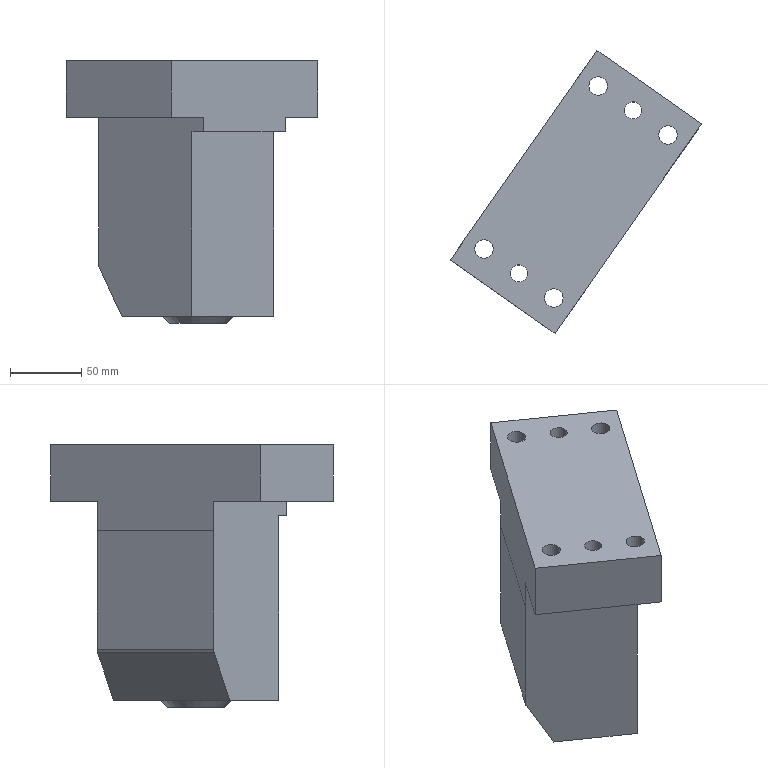Part | NX | features solid 2 | 1 solid | 34 faces | box 176.967 x 199.069 x 185 mm | volume 1701665 mm3 | plane 20 | cylinder 12 | cone 2 | commonest cylinder face diameters 20 x5 13 x4 12 x2 10 x1
STEP:
#1=CARTESIAN_POINT('',(-203.117,147.18,-70.));
#2=VERTEX_POINT('',#1);
#3=CARTESIAN_POINT('',(-196.617,147.18,-70.));
#4=DIRECTION('',(0.,0.,-1.));
#5=DIRECTION('',(-1.,0.,0.));
#6=AXIS2_PLACEMENT_3D('',#3,#4,#5);
#7=CIRCLE('',#6,6.5);
#8=EDGE_CURVE('',#2,#2,#7,.T.);
#9=ORIENTED_EDGE('',*,*,#8,.T.);
#10=EDGE_LOOP('',(#9));
#11=FACE_BOUND('',#10,.T.);
#12=CARTESIAN_POINT('',(-252.266,181.595,-70.));
#13=VERTEX_POINT('',#12);
#14=CARTESIAN_POINT('',(-245.766,181.595,-70.));
#15=DIRECTION('',(0.,0.,-1.));
#16=DIRECTION('',(-1.,0.,0.));
#17=AXIS2_PLACEMENT_3D('',#14,#15,#16);
#18=CIRCLE('',#17,6.5);
#19=EDGE_CURVE('',#13,#13,#18,.T.);
#20=ORIENTED_EDGE('',*,*,#19,.T.);
#21=EDGE_LOOP('',(#20));
#22=FACE_BOUND('',#21,.T.);
#23=CARTESIAN_POINT('',(-283.417,32.499,-70.));
#24=VERTEX_POINT('',#23);
#25=CARTESIAN_POINT('',(-276.917,32.499,-70.));
#26=DIRECTION('',(0.,0.,-1.));
#27=DIRECTION('',(-1.,0.,0.));
#28=AXIS2_PLACEMENT_3D('',#25,#26,#27);
#29=CIRCLE('',#28,6.5);
#30=EDGE_CURVE('',#24,#24,#29,.T.);
#31=ORIENTED_EDGE('',*,*,#30,.T.);
#32=EDGE_LOOP('',(#31));
#33=FACE_BOUND('',#32,.T.);
#34=CARTESIAN_POINT('',(-332.566,66.914,-70.));
#35=VERTEX_POINT('',#34);
#36=CARTESIAN_POINT('',(-326.066,66.914,-70.));
#37=DIRECTION('',(0.,0.,-1.));
#38=DIRECTION('',(-1.,0.,0.));
#39=AXIS2_PLACEMENT_3D('',#36,#37,#38);
#40=CIRCLE('',#39,6.5);
#41=EDGE_CURVE('',#35,#35,#40,.T.);
#42=ORIENTED_EDGE('',*,*,#41,.T.);
#43=EDGE_LOOP('',(#42));
#44=FACE_BOUND('',#43,.T.);
#45=CARTESIAN_POINT('',(-246.581,206.581,-70.));
#46=VERTEX_POINT('',#45);
#47=CARTESIAN_POINT('',(-349.824,59.134,-70.));
#48=VERTEX_POINT('',#47);
#49=CARTESIAN_POINT('',(-326.881,91.9,-70.));
#50=DIRECTION('',(-0.5736,-0.8192,0.));
#51=VECTOR('',#50,1000.);
#52=LINE('',#49,#51);
#53=EDGE_CURVE('',#46,#48,#52,.T.);
#54=ORIENTED_EDGE('',*,*,#53,.T.);
#55=CARTESIAN_POINT('',(-276.102,7.513,-70.));
#56=VERTEX_POINT('',#55);
#57=CARTESIAN_POINT('',(-349.825,59.134,-70.));
#58=DIRECTION('',(0.8192,-0.5736,0.));
#59=VECTOR('',#58,1000.);
#60=LINE('',#57,#59);
#61=EDGE_CURVE('',#48,#56,#60,.T.);
#62=ORIENTED_EDGE('',*,*,#61,.T.);
#63=CARTESIAN_POINT('',(-172.858,154.96,-70.));
#64=VERTEX_POINT('',#63);
#65=CARTESIAN_POINT('',(-253.159,40.279,-70.));
#66=DIRECTION('',(0.5736,0.8192,0.));
#67=VECTOR('',#66,1000.);
#68=LINE('',#65,#67);
#69=EDGE_CURVE('',#56,#64,#68,.T.);
#70=ORIENTED_EDGE('',*,*,#69,.T.);
#71=CARTESIAN_POINT('',(-263.134,218.172,-70.));
#72=DIRECTION('',(0.8192,-0.5736,0.));
#73=VECTOR('',#72,1000.);
#74=LINE('',#71,#73);
#75=EDGE_CURVE('',#46,#64,#74,.T.);
#76=ORIENTED_EDGE('',*,*,#75,.F.);
#77=EDGE_LOOP('',(#54,#62,#70,#76));
#78=FACE_BOUND('',#77,.T.);
#79=CARTESIAN_POINT('',(-227.191,164.388,-70.));
#80=VERTEX_POINT('',#79);
#81=CARTESIAN_POINT('',(-221.191,164.388,-70.));
#82=DIRECTION('',(0.,0.,-1.));
#83=DIRECTION('',(-1.,0.,0.));
#84=AXIS2_PLACEMENT_3D('',#81,#82,#83);
#85=CIRCLE('',#84,6.);
#86=EDGE_CURVE('',#80,#80,#85,.T.);
#87=ORIENTED_EDGE('',*,*,#86,.T.);
#88=EDGE_LOOP('',(#87));
#89=FACE_BOUND('',#88,.T.);
#90=CARTESIAN_POINT('',(-307.492,49.706,-70.));
#91=VERTEX_POINT('',#90);
#92=CARTESIAN_POINT('',(-301.492,49.706,-70.));
#93=DIRECTION('',(0.,0.,-1.));
#94=DIRECTION('',(-1.,0.,0.));
#95=AXIS2_PLACEMENT_3D('',#92,#93,#94);
#96=CIRCLE('',#95,6.);
#97=EDGE_CURVE('',#91,#91,#96,.F.);
#98=ORIENTED_EDGE('',*,*,#97,.F.);
#99=EDGE_LOOP('',(#98));
#100=FACE_BOUND('',#99,.T.);
#101=CARTESIAN_POINT('',(-343.435,103.491,-70.));
#102=DIRECTION('',(0.,0.,1.));
#103=DIRECTION('',(0.5736,0.8192,0.));
#104=AXIS2_PLACEMENT_3D('',#101,#102,#103);
#105=PLANE('',#104);
#106=ADVANCED_FACE('',(#11,#22,#33,#44,#78,#89,#100),#105,.T.);
#107=CARTESIAN_POINT('',(-286.917,32.499,-110.));
#108=VERTEX_POINT('',#107);
#109=CARTESIAN_POINT('',(-276.917,32.499,-110.));
#110=DIRECTION('',(0.,0.,-1.));
#111=DIRECTION('',(-1.,0.,0.));
#112=AXIS2_PLACEMENT_3D('',#109,#110,#111);
#113=CIRCLE('',#112,10.);
#114=EDGE_CURVE('',#108,#108,#113,.T.);
#115=ORIENTED_EDGE('',*,*,#114,.F.);
#116=EDGE_LOOP('',(#115));
#117=FACE_BOUND('',#116,.T.);
#118=CARTESIAN_POINT('',(-336.066,66.914,-110.));
#119=VERTEX_POINT('',#118);
#120=CARTESIAN_POINT('',(-326.066,66.914,-110.));
#121=DIRECTION('',(0.,0.,-1.));
#122=DIRECTION('',(-1.,0.,0.));
#123=AXIS2_PLACEMENT_3D('',#120,#121,#122);
#124=CIRCLE('',#123,10.);
#125=EDGE_CURVE('',#119,#119,#124,.T.);
#126=ORIENTED_EDGE('',*,*,#125,.F.);
#127=EDGE_LOOP('',(#126));
#128=FACE_BOUND('',#127,.T.);
#129=CARTESIAN_POINT('',(-326.881,91.9,-110.));
#130=VERTEX_POINT('',#129);
#131=CARTESIAN_POINT('',(-253.159,40.279,-110.));
#132=VERTEX_POINT('',#131);
#133=CARTESIAN_POINT('',(-326.882,91.9,-110.));
#134=DIRECTION('',(-0.8192,0.5736,0.));
#135=VECTOR('',#134,1000.);
#136=LINE('',#133,#135);
#137=EDGE_CURVE('',#130,#132,#136,.F.);
#138=ORIENTED_EDGE('',*,*,#137,.T.);
#139=CARTESIAN_POINT('',(-276.102,7.513,-110.));
#140=VERTEX_POINT('',#139);
#141=CARTESIAN_POINT('',(-253.159,40.279,-110.));
#142=DIRECTION('',(0.5736,0.8192,0.));
#143=VECTOR('',#142,1000.);
#144=LINE('',#141,#143);
#145=EDGE_CURVE('',#140,#132,#144,.T.);
#146=ORIENTED_EDGE('',*,*,#145,.F.);
#147=CARTESIAN_POINT('',(-349.824,59.134,-110.));
#148=VERTEX_POINT('',#147);
#149=CARTESIAN_POINT('',(-349.825,59.134,-110.));
#150=DIRECTION('',(0.8192,-0.5736,0.));
#151=VECTOR('',#150,1000.);
#152=LINE('',#149,#151);
#153=EDGE_CURVE('',#148,#140,#152,.T.);
#154=ORIENTED_EDGE('',*,*,#153,.F.);
#155=CARTESIAN_POINT('',(-326.881,91.9,-110.));
#156=DIRECTION('',(-0.5736,-0.8192,0.));
#157=VECTOR('',#156,1000.);
#158=LINE('',#155,#157);
#159=EDGE_CURVE('',#130,#148,#158,.T.);
#160=ORIENTED_EDGE('',*,*,#159,.F.);
#161=EDGE_LOOP('',(#138,#146,#154,#160));
#162=FACE_BOUND('',#161,.T.);
#163=CARTESIAN_POINT('',(-307.492,49.706,-110.));
#164=VERTEX_POINT('',#163);
#165=CARTESIAN_POINT('',(-301.492,49.706,-110.));
#166=DIRECTION('',(0.,0.,-1.));
#167=DIRECTION('',(-1.,0.,0.));
#168=AXIS2_PLACEMENT_3D('',#165,#166,#167);
#169=CIRCLE('',#168,6.);
#170=EDGE_CURVE('',#164,#164,#169,.F.);
#171=ORIENTED_EDGE('',*,*,#170,.T.);
#172=EDGE_LOOP('',(#171));
#173=FACE_BOUND('',#172,.T.);
#174=CARTESIAN_POINT('',(-343.435,103.491,-110.));
#175=DIRECTION('',(0.,0.,1.));
#176=DIRECTION('',(0.5736,0.8192,0.));
#177=AXIS2_PLACEMENT_3D('',#174,#175,#176);
#178=PLANE('',#177);
#179=ADVANCED_FACE('',(#117,#128,#162,#173),#178,.F.);
#180=CARTESIAN_POINT('',(-269.525,173.816,-130.5));
#181=VERTEX_POINT('',#180);
#182=CARTESIAN_POINT('',(-269.525,173.816,-214.019));
#183=VERTEX_POINT('',#182);
#184=CARTESIAN_POINT('',(-269.525,173.816,-200.));
#185=DIRECTION('',(0.,0.,-1.));
#186=VECTOR('',#185,1000.);
#187=LINE('',#184,#186);
#188=EDGE_CURVE('',#181,#183,#187,.T.);
#189=ORIENTED_EDGE('',*,*,#188,.F.);
#190=CARTESIAN_POINT('',(-269.524,173.815,-130.5));
#191=VERTEX_POINT('',#190);
#192=CARTESIAN_POINT('',(-269.525,173.816,-130.5));
#193=DIRECTION('',(-0.8192,0.5736,0.));
#194=VECTOR('',#193,1000.);
#195=LINE('',#192,#194);
#196=EDGE_CURVE('',#181,#191,#195,.F.);
#197=ORIENTED_EDGE('',*,*,#196,.T.);
#198=CARTESIAN_POINT('',(-269.524,173.815,-110.));
#199=VERTEX_POINT('',#198);
#200=CARTESIAN_POINT('',(-269.524,173.815,-130.));
#201=DIRECTION('',(0.,0.,1.));
#202=VECTOR('',#201,1000.);
#203=LINE('',#200,#202);
#204=EDGE_CURVE('',#191,#199,#203,.T.);
#205=ORIENTED_EDGE('',*,*,#204,.T.);
#206=CARTESIAN_POINT('',(-195.801,122.194,-110.));
#207=VERTEX_POINT('',#206);
#208=CARTESIAN_POINT('',(-269.525,173.816,-110.));
#209=DIRECTION('',(-0.8192,0.5736,0.));
#210=VECTOR('',#209,1000.);
#211=LINE('',#208,#210);
#212=EDGE_CURVE('',#207,#199,#211,.T.);
#213=ORIENTED_EDGE('',*,*,#212,.F.);
#214=CARTESIAN_POINT('',(-195.801,122.194,-120.));
#215=VERTEX_POINT('',#214);
#216=CARTESIAN_POINT('',(-195.801,122.194,-260.));
#217=DIRECTION('',(0.,0.,-1.));
#218=VECTOR('',#217,1000.);
#219=LINE('',#216,#218);
#220=EDGE_CURVE('',#207,#215,#219,.T.);
#221=ORIENTED_EDGE('',*,*,#220,.T.);
#222=CARTESIAN_POINT('',(-203.992,127.93,-120.));
#223=VERTEX_POINT('',#222);
#224=CARTESIAN_POINT('',(-269.525,173.816,-120.));
#225=DIRECTION('',(-0.8192,0.5736,0.));
#226=VECTOR('',#225,1000.);
#227=LINE('',#224,#226);
#228=EDGE_CURVE('',#215,#223,#227,.T.);
#229=ORIENTED_EDGE('',*,*,#228,.T.);
#230=CARTESIAN_POINT('',(-203.992,127.93,-250.));
#231=VERTEX_POINT('',#230);
#232=CARTESIAN_POINT('',(-203.992,127.93,-130.));
#233=DIRECTION('',(0.,0.,-1.));
#234=VECTOR('',#233,1000.);
#235=LINE('',#232,#234);
#236=EDGE_CURVE('',#223,#231,#235,.T.);
#237=ORIENTED_EDGE('',*,*,#236,.T.);
#238=CARTESIAN_POINT('',(-253.142,162.344,-250.));
#239=VERTEX_POINT('',#238);
#240=CARTESIAN_POINT('',(-269.525,173.816,-250.));
#241=DIRECTION('',(0.8192,-0.5736,0.));
#242=VECTOR('',#241,1000.);
#243=LINE('',#240,#242);
#244=EDGE_CURVE('',#239,#231,#243,.T.);
#245=ORIENTED_EDGE('',*,*,#244,.F.);
#246=CARTESIAN_POINT('',(-268.976,173.431,-216.519));
#247=VERTEX_POINT('',#246);
#248=CARTESIAN_POINT('',(-321.084,209.918,-106.34));
#249=DIRECTION('',(0.4096,-0.2868,-0.866));
#250=VECTOR('',#249,1000.);
#251=LINE('',#248,#250);
#252=EDGE_CURVE('',#247,#239,#251,.T.);
#253=ORIENTED_EDGE('',*,*,#252,.F.);
#254=CARTESIAN_POINT('',(-265.429,170.948,-214.019));
#255=DIRECTION('',(-0.5736,-0.8192,0.));
#256=DIRECTION('',(0.8192,-0.5736,0.));
#257=AXIS2_PLACEMENT_3D('',#254,#255,#256);
#258=CIRCLE('',#257,5.);
#259=EDGE_CURVE('',#183,#247,#258,.T.);
#260=ORIENTED_EDGE('',*,*,#259,.F.);
#261=EDGE_LOOP('',(#189,#197,#205,#213,#221,#229,#237,#245,#253,#260));
#262=FACE_BOUND('',#261,.T.);
#263=CARTESIAN_POINT('',(-269.525,173.816,-130.));
#264=DIRECTION('',(0.5736,0.8192,0.));
#265=DIRECTION('',(0.,0.,-1.));
#266=AXIS2_PLACEMENT_3D('',#263,#264,#265);
#267=PLANE('',#266);
#268=ADVANCED_FACE('',(#262),#267,.T.);
#269=CARTESIAN_POINT('',(-310.499,80.429,-250.));
#270=VERTEX_POINT('',#269);
#271=CARTESIAN_POINT('',(-326.334,91.516,-216.519));
#272=VERTEX_POINT('',#271);
#273=CARTESIAN_POINT('',(-378.442,128.003,-106.34));
#274=DIRECTION('',(0.4096,-0.2868,-0.866));
#275=VECTOR('',#274,1000.);
#276=LINE('',#273,#275);
#277=EDGE_CURVE('',#270,#272,#276,.F.);
#278=ORIENTED_EDGE('',*,*,#277,.F.);
#279=CARTESIAN_POINT('',(-261.35,46.014,-250.));
#280=VERTEX_POINT('',#279);
#281=CARTESIAN_POINT('',(-351.457,109.108,-250.));
#282=DIRECTION('',(-0.8192,0.5736,0.));
#283=VECTOR('',#282,1000.);
#284=LINE('',#281,#283);
#285=EDGE_CURVE('',#270,#280,#284,.F.);
#286=ORIENTED_EDGE('',*,*,#285,.T.);
#287=CARTESIAN_POINT('',(-261.35,46.014,-120.));
#288=VERTEX_POINT('',#287);
#289=CARTESIAN_POINT('',(-261.35,46.014,-130.));
#290=DIRECTION('',(0.,0.,-1.));
#291=VECTOR('',#290,1000.);
#292=LINE('',#289,#291);
#293=EDGE_CURVE('',#280,#288,#292,.F.);
#294=ORIENTED_EDGE('',*,*,#293,.T.);
#295=CARTESIAN_POINT('',(-253.159,40.279,-120.));
#296=VERTEX_POINT('',#295);
#297=CARTESIAN_POINT('',(-326.882,91.9,-120.));
#298=DIRECTION('',(-0.8192,0.5736,0.));
#299=VECTOR('',#298,1000.);
#300=LINE('',#297,#299);
#301=EDGE_CURVE('',#288,#296,#300,.F.);
#302=ORIENTED_EDGE('',*,*,#301,.T.);
#303=CARTESIAN_POINT('',(-253.159,40.279,-260.));
#304=DIRECTION('',(0.,0.,-1.));
#305=VECTOR('',#304,1000.);
#306=LINE('',#303,#305);
#307=EDGE_CURVE('',#296,#132,#306,.F.);
#308=ORIENTED_EDGE('',*,*,#307,.T.);
#309=ORIENTED_EDGE('',*,*,#137,.F.);
#310=CARTESIAN_POINT('',(-326.881,91.9,-130.5));
#311=VERTEX_POINT('',#310);
#312=CARTESIAN_POINT('',(-326.881,91.9,-130.));
#313=DIRECTION('',(0.,0.,1.));
#314=VECTOR('',#313,1000.);
#315=LINE('',#312,#314);
#316=EDGE_CURVE('',#130,#311,#315,.F.);
#317=ORIENTED_EDGE('',*,*,#316,.T.);
#318=CARTESIAN_POINT('',(-326.882,91.9,-130.5));
#319=VERTEX_POINT('',#318);
#320=CARTESIAN_POINT('',(-326.882,91.9,-130.5));
#321=DIRECTION('',(-0.8192,0.5736,0.));
#322=VECTOR('',#321,1000.);
#323=LINE('',#320,#322);
#324=EDGE_CURVE('',#311,#319,#323,.T.);
#325=ORIENTED_EDGE('',*,*,#324,.T.);
#326=CARTESIAN_POINT('',(-326.882,91.9,-214.019));
#327=VERTEX_POINT('',#326);
#328=CARTESIAN_POINT('',(-326.882,91.9,-200.));
#329=DIRECTION('',(0.,0.,-1.));
#330=VECTOR('',#329,1000.);
#331=LINE('',#328,#330);
#332=EDGE_CURVE('',#327,#319,#331,.F.);
#333=ORIENTED_EDGE('',*,*,#332,.F.);
#334=CARTESIAN_POINT('',(-322.786,89.033,-214.019));
#335=DIRECTION('',(-0.5736,-0.8192,0.));
#336=DIRECTION('',(0.8192,-0.5736,0.));
#337=AXIS2_PLACEMENT_3D('',#334,#335,#336);
#338=CIRCLE('',#337,5.);
#339=EDGE_CURVE('',#272,#327,#338,.F.);
#340=ORIENTED_EDGE('',*,*,#339,.F.);
#341=EDGE_LOOP('',(#278,#286,#294,#302,#308,#309,#317,#325,#333,#340));
#342=FACE_BOUND('',#341,.T.);
#343=CARTESIAN_POINT('',(-326.882,91.9,-130.));
#344=DIRECTION('',(0.5736,0.8192,0.));
#345=DIRECTION('',(0.,0.,-1.));
#346=AXIS2_PLACEMENT_3D('',#343,#344,#345);
#347=PLANE('',#346);
#348=ADVANCED_FACE('',(#342),#347,.F.);
#349=CARTESIAN_POINT('',(-232.626,108.52,-250.));
#350=VERTEX_POINT('',#349);
#351=CARTESIAN_POINT('',(-257.246,104.179,-250.));
#352=DIRECTION('',(0.,0.,1.));
#353=DIRECTION('',(0.9848,0.1736,0.));
#354=AXIS2_PLACEMENT_3D('',#351,#352,#353);
#355=CIRCLE('',#354,25.);
#356=EDGE_CURVE('',#350,#350,#355,.F.);
#357=ORIENTED_EDGE('',*,*,#356,.F.);
#358=EDGE_LOOP('',(#357));
#359=FACE_BOUND('',#358,.T.);
#360=CARTESIAN_POINT('',(-261.35,46.014,-250.));
#361=DIRECTION('',(-0.5736,-0.8192,0.));
#362=VECTOR('',#361,1000.);
#363=LINE('',#360,#362);
#364=EDGE_CURVE('',#231,#280,#363,.T.);
#365=ORIENTED_EDGE('',*,*,#364,.T.);
#366=ORIENTED_EDGE('',*,*,#285,.F.);
#367=CARTESIAN_POINT('',(-310.499,80.429,-250.));
#368=DIRECTION('',(-0.5736,-0.8192,0.));
#369=VECTOR('',#368,1000.);
#370=LINE('',#367,#369);
#371=EDGE_CURVE('',#239,#270,#370,.T.);
#372=ORIENTED_EDGE('',*,*,#371,.F.);
#373=ORIENTED_EDGE('',*,*,#244,.T.);
#374=EDGE_LOOP('',(#365,#366,#372,#373));
#375=FACE_BOUND('',#374,.T.);
#376=CARTESIAN_POINT('',(-351.457,109.108,-250.));
#377=DIRECTION('',(0.,0.,-1.));
#378=DIRECTION('',(-0.5736,-0.8192,0.));
#379=AXIS2_PLACEMENT_3D('',#376,#377,#378);
#380=PLANE('',#379);
#381=ADVANCED_FACE('',(#359,#375),#380,.T.);
#382=ORIENTED_EDGE('',*,*,#332,.T.);
#383=CARTESIAN_POINT('',(-326.882,91.9,-130.5));
#384=DIRECTION('',(0.5736,0.8192,0.));
#385=VECTOR('',#384,1000.);
#386=LINE('',#383,#385);
#387=EDGE_CURVE('',#181,#319,#386,.F.);
#388=ORIENTED_EDGE('',*,*,#387,.F.);
#389=ORIENTED_EDGE('',*,*,#188,.T.);
#390=CARTESIAN_POINT('',(-269.525,173.816,-214.019));
#391=DIRECTION('',(0.5736,0.8192,0.));
#392=VECTOR('',#391,1000.);
#393=LINE('',#390,#392);
#394=EDGE_CURVE('',#327,#183,#393,.T.);
#395=ORIENTED_EDGE('',*,*,#394,.F.);
#396=EDGE_LOOP('',(#382,#388,#389,#395));
#397=FACE_BOUND('',#396,.T.);
#398=CARTESIAN_POINT('',(-326.882,91.9,-200.));
#399=DIRECTION('',(0.8192,-0.5736,0.));
#400=DIRECTION('',(-0.5736,-0.8192,0.));
#401=AXIS2_PLACEMENT_3D('',#398,#399,#400);
#402=PLANE('',#401);
#403=ADVANCED_FACE('',(#397),#402,.F.);
#404=CARTESIAN_POINT('',(-253.159,40.279,-120.));
#405=DIRECTION('',(0.5736,0.8192,0.));
#406=VECTOR('',#405,1000.);
#407=LINE('',#404,#406);
#408=EDGE_CURVE('',#296,#215,#407,.T.);
#409=ORIENTED_EDGE('',*,*,#408,.T.);
#410=ORIENTED_EDGE('',*,*,#220,.F.);
#411=CARTESIAN_POINT('',(-172.858,154.96,-110.));
#412=VERTEX_POINT('',#411);
#413=CARTESIAN_POINT('',(-253.159,40.279,-110.));
#414=DIRECTION('',(0.5736,0.8192,0.));
#415=VECTOR('',#414,1000.);
#416=LINE('',#413,#415);
#417=EDGE_CURVE('',#207,#412,#416,.T.);
#418=ORIENTED_EDGE('',*,*,#417,.T.);
#419=CARTESIAN_POINT('',(-172.858,154.96,-90.));
#420=DIRECTION('',(0.,0.,-1.));
#421=VECTOR('',#420,1000.);
#422=LINE('',#419,#421);
#423=EDGE_CURVE('',#64,#412,#422,.T.);
#424=ORIENTED_EDGE('',*,*,#423,.F.);
#425=ORIENTED_EDGE('',*,*,#69,.F.);
#426=CARTESIAN_POINT('',(-276.102,7.513,-90.));
#427=DIRECTION('',(0.,0.,-1.));
#428=VECTOR('',#427,1000.);
#429=LINE('',#426,#428);
#430=EDGE_CURVE('',#56,#140,#429,.T.);
#431=ORIENTED_EDGE('',*,*,#430,.T.);
#432=ORIENTED_EDGE('',*,*,#145,.T.);
#433=ORIENTED_EDGE('',*,*,#307,.F.);
#434=EDGE_LOOP('',(#409,#410,#418,#424,#425,#431,#432,#433));
#435=FACE_BOUND('',#434,.T.);
#436=CARTESIAN_POINT('',(-253.159,40.279,-260.));
#437=DIRECTION('',(0.8192,-0.5736,0.));
#438=DIRECTION('',(-0.5736,-0.8192,0.));
#439=AXIS2_PLACEMENT_3D('',#436,#437,#438);
#440=PLANE('',#439);
#441=ADVANCED_FACE('',(#435),#440,.T.);
#442=ORIENTED_EDGE('',*,*,#252,.T.);
#443=ORIENTED_EDGE('',*,*,#371,.T.);
#444=ORIENTED_EDGE('',*,*,#277,.T.);
#445=CARTESIAN_POINT('',(-326.334,91.516,-216.519));
#446=DIRECTION('',(0.5736,0.8192,0.));
#447=VECTOR('',#446,1000.);
#448=LINE('',#445,#447);
#449=EDGE_CURVE('',#247,#272,#448,.F.);
#450=ORIENTED_EDGE('',*,*,#449,.F.);
#451=EDGE_LOOP('',(#442,#443,#444,#450));
#452=FACE_BOUND('',#451,.T.);
#453=CARTESIAN_POINT('',(-326.882,91.9,-215.359));
#454=DIRECTION('',(-0.7094,0.4967,-0.5));
#455=DIRECTION('',(0.5736,0.8192,0.));
#456=AXIS2_PLACEMENT_3D('',#453,#454,#455);
#457=PLANE('',#456);
#458=ADVANCED_FACE('',(#452),#457,.T.);
#459=CARTESIAN_POINT('',(-349.824,59.134,-30.5));
#460=DIRECTION('',(0.,0.,1.));
#461=VECTOR('',#460,1000.);
#462=LINE('',#459,#461);
#463=EDGE_CURVE('',#48,#148,#462,.F.);
#464=ORIENTED_EDGE('',*,*,#463,.T.);
#465=ORIENTED_EDGE('',*,*,#153,.T.);
#466=ORIENTED_EDGE('',*,*,#430,.F.);
#467=ORIENTED_EDGE('',*,*,#61,.F.);
#468=EDGE_LOOP('',(#464,#465,#466,#467));
#469=FACE_BOUND('',#468,.T.);
#470=CARTESIAN_POINT('',(-349.825,59.134,-90.));
#471=DIRECTION('',(-0.5736,-0.8192,0.));
#472=DIRECTION('',(-0.8192,0.5736,0.));
#473=AXIS2_PLACEMENT_3D('',#470,#471,#472);
#474=PLANE('',#473);
#475=ADVANCED_FACE('',(#469),#474,.T.);
#476=CARTESIAN_POINT('',(-206.617,147.18,-110.));
#477=VERTEX_POINT('',#476);
#478=CARTESIAN_POINT('',(-196.617,147.18,-110.));
#479=DIRECTION('',(0.,0.,-1.));
#480=DIRECTION('',(-1.,0.,0.));
#481=AXIS2_PLACEMENT_3D('',#478,#479,#480);
#482=CIRCLE('',#481,10.);
#483=EDGE_CURVE('',#477,#477,#482,.T.);
#484=ORIENTED_EDGE('',*,*,#483,.F.);
#485=EDGE_LOOP('',(#484));
#486=FACE_BOUND('',#485,.T.);
#487=CARTESIAN_POINT('',(-255.766,181.595,-110.));
#488=VERTEX_POINT('',#487);
#489=CARTESIAN_POINT('',(-245.766,181.595,-110.));
#490=DIRECTION('',(0.,0.,-1.));
#491=DIRECTION('',(-1.,0.,0.));
#492=AXIS2_PLACEMENT_3D('',#489,#490,#491);
#493=CIRCLE('',#492,10.);
#494=EDGE_CURVE('',#488,#488,#493,.T.);
#495=ORIENTED_EDGE('',*,*,#494,.F.);
#496=EDGE_LOOP('',(#495));
#497=FACE_BOUND('',#496,.T.);
#498=CARTESIAN_POINT('',(-227.191,164.388,-110.));
#499=VERTEX_POINT('',#498);
#500=CARTESIAN_POINT('',(-221.191,164.388,-110.));
#501=DIRECTION('',(0.,0.,-1.));
#502=DIRECTION('',(-1.,0.,0.));
#503=AXIS2_PLACEMENT_3D('',#500,#501,#502);
#504=CIRCLE('',#503,6.);
#505=EDGE_CURVE('',#499,#499,#504,.T.);
#506=ORIENTED_EDGE('',*,*,#505,.F.);
#507=EDGE_LOOP('',(#506));
#508=FACE_BOUND('',#507,.T.);
#509=CARTESIAN_POINT('',(-246.581,206.581,-110.));
#510=VERTEX_POINT('',#509);
#511=CARTESIAN_POINT('',(-263.134,218.172,-110.));
#512=DIRECTION('',(0.8192,-0.5736,0.));
#513=VECTOR('',#512,1000.);
#514=LINE('',#511,#513);
#515=EDGE_CURVE('',#510,#412,#514,.T.);
#516=ORIENTED_EDGE('',*,*,#515,.T.);
#517=ORIENTED_EDGE('',*,*,#417,.F.);
#518=ORIENTED_EDGE('',*,*,#212,.T.);
#519=CARTESIAN_POINT('',(-326.881,91.9,-110.));
#520=DIRECTION('',(-0.5736,-0.8192,0.));
#521=VECTOR('',#520,1000.);
#522=LINE('',#519,#521);
#523=EDGE_CURVE('',#510,#199,#522,.T.);
#524=ORIENTED_EDGE('',*,*,#523,.F.);
#525=EDGE_LOOP('',(#516,#517,#518,#524));
#526=FACE_BOUND('',#525,.T.);
#527=CARTESIAN_POINT('',(-343.435,103.491,-110.));
#528=DIRECTION('',(0.,0.,1.));
#529=DIRECTION('',(0.5736,0.8192,0.));
#530=AXIS2_PLACEMENT_3D('',#527,#528,#529);
#531=PLANE('',#530);
#532=ADVANCED_FACE('',(#486,#497,#508,#526),#531,.F.);
#533=ORIENTED_EDGE('',*,*,#75,.T.);
#534=ORIENTED_EDGE('',*,*,#423,.T.);
#535=ORIENTED_EDGE('',*,*,#515,.F.);
#536=CARTESIAN_POINT('',(-246.581,206.581,-30.5));
#537=DIRECTION('',(0.,0.,1.));
#538=VECTOR('',#537,1000.);
#539=LINE('',#536,#538);
#540=EDGE_CURVE('',#46,#510,#539,.F.);
#541=ORIENTED_EDGE('',*,*,#540,.F.);
#542=EDGE_LOOP('',(#533,#534,#535,#541));
#543=FACE_BOUND('',#542,.T.);
#544=CARTESIAN_POINT('',(-263.134,218.172,-90.));
#545=DIRECTION('',(-0.5736,-0.8192,0.));
#546=DIRECTION('',(-0.8192,0.5736,0.));
#547=AXIS2_PLACEMENT_3D('',#544,#545,#546);
#548=PLANE('',#547);
#549=ADVANCED_FACE('',(#543),#548,.F.);
#550=ORIENTED_EDGE('',*,*,#228,.F.);
#551=ORIENTED_EDGE('',*,*,#408,.F.);
#552=ORIENTED_EDGE('',*,*,#301,.F.);
#553=CARTESIAN_POINT('',(-261.35,46.014,-120.));
#554=DIRECTION('',(0.5736,0.8192,0.));
#555=VECTOR('',#554,1000.);
#556=LINE('',#553,#555);
#557=EDGE_CURVE('',#288,#223,#556,.T.);
#558=ORIENTED_EDGE('',*,*,#557,.T.);
#559=EDGE_LOOP('',(#550,#551,#552,#558));
#560=FACE_BOUND('',#559,.T.);
#561=CARTESIAN_POINT('',(-261.35,46.014,-120.));
#562=DIRECTION('',(0.,0.,1.));
#563=DIRECTION('',(0.1736,-0.9848,0.));
#564=AXIS2_PLACEMENT_3D('',#561,#562,#563);
#565=PLANE('',#564);
#566=ADVANCED_FACE('',(#560),#565,.F.);
#567=ORIENTED_EDGE('',*,*,#236,.F.);
#568=ORIENTED_EDGE('',*,*,#557,.F.);
#569=ORIENTED_EDGE('',*,*,#293,.F.);
#570=ORIENTED_EDGE('',*,*,#364,.F.);
#571=EDGE_LOOP('',(#567,#568,#569,#570));
#572=FACE_BOUND('',#571,.T.);
#573=CARTESIAN_POINT('',(-261.35,46.014,-250.));
#574=DIRECTION('',(-0.8192,0.5736,0.));
#575=DIRECTION('',(0.,0.,-1.));
#576=AXIS2_PLACEMENT_3D('',#573,#574,#575);
#577=PLANE('',#576);
#578=ADVANCED_FACE('',(#572),#577,.F.);
#579=ORIENTED_EDGE('',*,*,#196,.F.);
#580=ORIENTED_EDGE('',*,*,#387,.T.);
#581=ORIENTED_EDGE('',*,*,#324,.F.);
#582=CARTESIAN_POINT('',(-349.824,59.134,-130.5));
#583=DIRECTION('',(-0.5736,-0.8192,0.));
#584=VECTOR('',#583,1000.);
#585=LINE('',#582,#584);
#586=EDGE_CURVE('',#311,#191,#585,.F.);
#587=ORIENTED_EDGE('',*,*,#586,.T.);
#588=EDGE_LOOP('',(#579,#580,#581,#587));
#589=FACE_BOUND('',#588,.T.);
#590=CARTESIAN_POINT('',(-349.825,59.134,-130.5));
#591=DIRECTION('',(0.,0.,1.));
#592=DIRECTION('',(0.5736,0.8192,0.));
#593=AXIS2_PLACEMENT_3D('',#590,#591,#592);
#594=PLANE('',#593);
#595=ADVANCED_FACE('',(#589),#594,.T.);
#596=ORIENTED_EDGE('',*,*,#53,.F.);
#597=ORIENTED_EDGE('',*,*,#540,.T.);
#598=ORIENTED_EDGE('',*,*,#523,.T.);
#599=ORIENTED_EDGE('',*,*,#204,.F.);
#600=ORIENTED_EDGE('',*,*,#586,.F.);
#601=ORIENTED_EDGE('',*,*,#316,.F.);
#602=ORIENTED_EDGE('',*,*,#159,.T.);
#603=ORIENTED_EDGE('',*,*,#463,.F.);
#604=EDGE_LOOP('',(#596,#597,#598,#599,#600,#601,#602,#603));
#605=FACE_BOUND('',#604,.T.);
#606=CARTESIAN_POINT('',(-349.824,59.134,-30.5));
#607=DIRECTION('',(0.8192,-0.5736,0.));
#608=DIRECTION('',(-0.5736,-0.8192,0.));
#609=AXIS2_PLACEMENT_3D('',#606,#607,#608);
#610=PLANE('',#609);
#611=ADVANCED_FACE('',(#605),#610,.F.);
#612=ORIENTED_EDGE('',*,*,#339,.T.);
#613=ORIENTED_EDGE('',*,*,#394,.T.);
#614=ORIENTED_EDGE('',*,*,#259,.T.);
#615=ORIENTED_EDGE('',*,*,#449,.T.);
#616=EDGE_LOOP('',(#612,#613,#614,#615));
#617=FACE_BOUND('',#616,.T.);
#618=CARTESIAN_POINT('',(-322.786,89.033,-214.019));
#619=DIRECTION('',(-0.5736,-0.8192,0.));
#620=DIRECTION('',(-0.8192,0.5736,0.));
#621=AXIS2_PLACEMENT_3D('',#618,#619,#620);
#622=CYLINDRICAL_SURFACE('',#621,5.);
#623=ADVANCED_FACE('',(#617),#622,.T.);
#624=CARTESIAN_POINT('',(-266.381,102.527,-255.));
#625=VERTEX_POINT('',#624);
#626=CARTESIAN_POINT('',(-256.532,104.263,-255.));
#627=DIRECTION('',(0.,0.,-1.));
#628=DIRECTION('',(-0.9848,-0.1736,0.));
#629=AXIS2_PLACEMENT_3D('',#626,#627,#628);
#630=CIRCLE('',#629,10.);
#631=EDGE_CURVE('',#625,#625,#630,.T.);
#632=ORIENTED_EDGE('',*,*,#631,.F.);
#633=EDGE_LOOP('',(#632));
#634=FACE_BOUND('',#633,.T.);
#635=CARTESIAN_POINT('',(-237.55,107.652,-255.));
#636=VERTEX_POINT('',#635);
#637=CARTESIAN_POINT('',(-257.246,104.179,-255.));
#638=DIRECTION('',(0.,0.,1.));
#639=DIRECTION('',(0.9848,0.1736,0.));
#640=AXIS2_PLACEMENT_3D('',#637,#638,#639);
#641=CIRCLE('',#640,20.);
#642=EDGE_CURVE('',#636,#636,#641,.T.);
#643=ORIENTED_EDGE('',*,*,#642,.F.);
#644=EDGE_LOOP('',(#643));
#645=FACE_BOUND('',#644,.T.);
#646=CARTESIAN_POINT('',(-257.246,104.179,-255.));
#647=DIRECTION('',(0.,0.,-1.));
#648=DIRECTION('',(0.9848,0.1736,0.));
#649=AXIS2_PLACEMENT_3D('',#646,#647,#648);
#650=PLANE('',#649);
#651=ADVANCED_FACE('',(#634,#645),#650,.T.);
#652=ORIENTED_EDGE('',*,*,#356,.T.);
#653=EDGE_LOOP('',(#652));
#654=FACE_BOUND('',#653,.T.);
#655=ORIENTED_EDGE('',*,*,#642,.T.);
#656=EDGE_LOOP('',(#655));
#657=FACE_BOUND('',#656,.T.);
#658=CARTESIAN_POINT('',(-257.246,104.179,-255.));
#659=DIRECTION('',(0.,0.,1.));
#660=DIRECTION('',(-0.9848,-0.1736,0.));
#661=AXIS2_PLACEMENT_3D('',#658,#659,#660);
#662=CONICAL_SURFACE('',#661,20.,0.7854);
#663=ADVANCED_FACE('',(#654,#657),#662,.T.);
#664=CARTESIAN_POINT('',(-266.381,102.527,-230.));
#665=VERTEX_POINT('',#664);
#666=CARTESIAN_POINT('',(-256.532,104.263,-230.));
#667=DIRECTION('',(0.,0.,-1.));
#668=DIRECTION('',(-0.9848,-0.1736,0.));
#669=AXIS2_PLACEMENT_3D('',#666,#667,#668);
#670=CIRCLE('',#669,10.);
#671=EDGE_CURVE('',#665,#665,#670,.T.);
#672=ORIENTED_EDGE('',*,*,#671,.T.);
#673=EDGE_LOOP('',(#672));
#674=FACE_BOUND('',#673,.T.);
#675=CARTESIAN_POINT('',(-256.532,104.263,-223.991));
#676=VERTEX_POINT('',#675);
#677=VERTEX_LOOP('',#676);
#678=FACE_BOUND('',#677,.T.);
#679=CARTESIAN_POINT('',(-256.532,104.263,-230.));
#680=DIRECTION('',(0.,0.,-1.));
#681=DIRECTION('',(0.9848,0.1736,0.));
#682=AXIS2_PLACEMENT_3D('',#679,#680,#681);
#683=CONICAL_SURFACE('',#682,10.,1.03);
#684=ADVANCED_FACE('',(#674,#678),#683,.F.);
#685=ORIENTED_EDGE('',*,*,#671,.F.);
#686=EDGE_LOOP('',(#685));
#687=FACE_BOUND('',#686,.T.);
#688=ORIENTED_EDGE('',*,*,#631,.T.);
#689=EDGE_LOOP('',(#688));
#690=FACE_BOUND('',#689,.T.);
#691=CARTESIAN_POINT('',(-256.532,104.263,-255.));
#692=DIRECTION('',(0.,0.,1.));
#693=DIRECTION('',(-0.9848,-0.1736,0.));
#694=AXIS2_PLACEMENT_3D('',#691,#692,#693);
#695=CYLINDRICAL_SURFACE('',#694,10.);
#696=ADVANCED_FACE('',(#687,#690),#695,.F.);
#697=ORIENTED_EDGE('',*,*,#86,.F.);
#698=EDGE_LOOP('',(#697));
#699=FACE_BOUND('',#698,.T.);
#700=ORIENTED_EDGE('',*,*,#505,.T.);
#701=EDGE_LOOP('',(#700));
#702=FACE_BOUND('',#701,.T.);
#703=CARTESIAN_POINT('',(-221.191,164.388,-210.));
#704=DIRECTION('',(0.,0.,1.));
#705=DIRECTION('',(-1.,0.,0.));
#706=AXIS2_PLACEMENT_3D('',#703,#704,#705);
#707=CYLINDRICAL_SURFACE('',#706,6.);
#708=ADVANCED_FACE('',(#699,#702),#707,.F.);
#709=ORIENTED_EDGE('',*,*,#97,.T.);
#710=EDGE_LOOP('',(#709));
#711=FACE_BOUND('',#710,.T.);
#712=ORIENTED_EDGE('',*,*,#170,.F.);
#713=EDGE_LOOP('',(#712));
#714=FACE_BOUND('',#713,.T.);
#715=CARTESIAN_POINT('',(-301.492,49.706,-210.));
#716=DIRECTION('',(0.,0.,1.));
#717=DIRECTION('',(-1.,0.,0.));
#718=AXIS2_PLACEMENT_3D('',#715,#716,#717);
#719=CYLINDRICAL_SURFACE('',#718,6.);
#720=ADVANCED_FACE('',(#711,#714),#719,.F.);
#721=CARTESIAN_POINT('',(-316.066,66.914,-95.));
#722=VERTEX_POINT('',#721);
#723=CARTESIAN_POINT('',(-326.066,66.914,-95.));
#724=DIRECTION('',(0.,0.,1.));
#725=DIRECTION('',(1.,0.,0.));
#726=AXIS2_PLACEMENT_3D('',#723,#724,#725);
#727=CIRCLE('',#726,10.);
#728=EDGE_CURVE('',#722,#722,#727,.T.);
#729=ORIENTED_EDGE('',*,*,#728,.T.);
#730=EDGE_LOOP('',(#729));
#731=FACE_BOUND('',#730,.T.);
#732=ORIENTED_EDGE('',*,*,#125,.T.);
#733=EDGE_LOOP('',(#732));
#734=FACE_BOUND('',#733,.T.);
#735=CARTESIAN_POINT('',(-326.066,66.914,-95.));
#736=DIRECTION('',(0.,0.,-1.));
#737=DIRECTION('',(1.,0.,0.));
#738=AXIS2_PLACEMENT_3D('',#735,#736,#737);
#739=CYLINDRICAL_SURFACE('',#738,10.);
#740=ADVANCED_FACE('',(#731,#734),#739,.F.);
#741=ORIENTED_EDGE('',*,*,#41,.F.);
#742=EDGE_LOOP('',(#741));
#743=FACE_BOUND('',#742,.T.);
#744=CARTESIAN_POINT('',(-332.566,66.914,-95.));
#745=VERTEX_POINT('',#744);
#746=CARTESIAN_POINT('',(-326.066,66.914,-95.));
#747=DIRECTION('',(0.,0.,-1.));
#748=DIRECTION('',(-1.,0.,0.));
#749=AXIS2_PLACEMENT_3D('',#746,#747,#748);
#750=CIRCLE('',#749,6.5);
#751=EDGE_CURVE('',#745,#745,#750,.F.);
#752=ORIENTED_EDGE('',*,*,#751,.F.);
#753=EDGE_LOOP('',(#752));
#754=FACE_BOUND('',#753,.T.);
#755=CARTESIAN_POINT('',(-326.066,66.914,-45.));
#756=DIRECTION('',(0.,0.,-1.));
#757=DIRECTION('',(1.,0.,0.));
#758=AXIS2_PLACEMENT_3D('',#755,#756,#757);
#759=CYLINDRICAL_SURFACE('',#758,6.5);
#760=ADVANCED_FACE('',(#743,#754),#759,.F.);
#761=ORIENTED_EDGE('',*,*,#751,.T.);
#762=EDGE_LOOP('',(#761));
#763=FACE_BOUND('',#762,.T.);
#764=ORIENTED_EDGE('',*,*,#728,.F.);
#765=EDGE_LOOP('',(#764));
#766=FACE_BOUND('',#765,.T.);
#767=CARTESIAN_POINT('',(-326.066,66.914,-95.));
#768=DIRECTION('',(0.,0.,1.));
#769=DIRECTION('',(-1.,0.,0.));
#770=AXIS2_PLACEMENT_3D('',#767,#768,#769);
#771=PLANE('',#770);
#772=ADVANCED_FACE('',(#763,#766),#771,.F.);
#773=CARTESIAN_POINT('',(-266.917,32.499,-95.));
#774=VERTEX_POINT('',#773);
#775=CARTESIAN_POINT('',(-276.917,32.499,-95.));
#776=DIRECTION('',(0.,0.,1.));
#777=DIRECTION('',(1.,0.,0.));
#778=AXIS2_PLACEMENT_3D('',#775,#776,#777);
#779=CIRCLE('',#778,10.);
#780=EDGE_CURVE('',#774,#774,#779,.T.);
#781=ORIENTED_EDGE('',*,*,#780,.T.);
#782=EDGE_LOOP('',(#781));
#783=FACE_BOUND('',#782,.T.);
#784=ORIENTED_EDGE('',*,*,#114,.T.);
#785=EDGE_LOOP('',(#784));
#786=FACE_BOUND('',#785,.T.);
#787=CARTESIAN_POINT('',(-276.917,32.499,-95.));
#788=DIRECTION('',(0.,0.,-1.));
#789=DIRECTION('',(1.,0.,0.));
#790=AXIS2_PLACEMENT_3D('',#787,#788,#789);
#791=CYLINDRICAL_SURFACE('',#790,10.);
#792=ADVANCED_FACE('',(#783,#786),#791,.F.);
#793=ORIENTED_EDGE('',*,*,#30,.F.);
#794=EDGE_LOOP('',(#793));
#795=FACE_BOUND('',#794,.T.);
#796=CARTESIAN_POINT('',(-283.417,32.499,-95.));
#797=VERTEX_POINT('',#796);
#798=CARTESIAN_POINT('',(-276.917,32.499,-95.));
#799=DIRECTION('',(0.,0.,-1.));
#800=DIRECTION('',(-1.,0.,0.));
#801=AXIS2_PLACEMENT_3D('',#798,#799,#800);
#802=CIRCLE('',#801,6.5);
#803=EDGE_CURVE('',#797,#797,#802,.F.);
#804=ORIENTED_EDGE('',*,*,#803,.F.);
#805=EDGE_LOOP('',(#804));
#806=FACE_BOUND('',#805,.T.);
#807=CARTESIAN_POINT('',(-276.917,32.499,-45.));
#808=DIRECTION('',(0.,0.,-1.));
#809=DIRECTION('',(1.,0.,0.));
#810=AXIS2_PLACEMENT_3D('',#807,#808,#809);
#811=CYLINDRICAL_SURFACE('',#810,6.5);
#812=ADVANCED_FACE('',(#795,#806),#811,.F.);
#813=ORIENTED_EDGE('',*,*,#803,.T.);
#814=EDGE_LOOP('',(#813));
#815=FACE_BOUND('',#814,.T.);
#816=ORIENTED_EDGE('',*,*,#780,.F.);
#817=EDGE_LOOP('',(#816));
#818=FACE_BOUND('',#817,.T.);
#819=CARTESIAN_POINT('',(-276.917,32.499,-95.));
#820=DIRECTION('',(0.,0.,1.));
#821=DIRECTION('',(-1.,0.,0.));
#822=AXIS2_PLACEMENT_3D('',#819,#820,#821);
#823=PLANE('',#822);
#824=ADVANCED_FACE('',(#815,#818),#823,.F.);
#825=CARTESIAN_POINT('',(-235.766,181.595,-95.));
#826=VERTEX_POINT('',#825);
#827=CARTESIAN_POINT('',(-245.766,181.595,-95.));
#828=DIRECTION('',(0.,0.,1.));
#829=DIRECTION('',(1.,0.,0.));
#830=AXIS2_PLACEMENT_3D('',#827,#828,#829);
#831=CIRCLE('',#830,10.);
#832=EDGE_CURVE('',#826,#826,#831,.T.);
#833=ORIENTED_EDGE('',*,*,#832,.T.);
#834=EDGE_LOOP('',(#833));
#835=FACE_BOUND('',#834,.T.);
#836=ORIENTED_EDGE('',*,*,#494,.T.);
#837=EDGE_LOOP('',(#836));
#838=FACE_BOUND('',#837,.T.);
#839=CARTESIAN_POINT('',(-245.766,181.595,-95.));
#840=DIRECTION('',(0.,0.,-1.));
#841=DIRECTION('',(1.,0.,0.));
#842=AXIS2_PLACEMENT_3D('',#839,#840,#841);
#843=CYLINDRICAL_SURFACE('',#842,10.);
#844=ADVANCED_FACE('',(#835,#838),#843,.F.);
#845=ORIENTED_EDGE('',*,*,#19,.F.);
#846=EDGE_LOOP('',(#845));
#847=FACE_BOUND('',#846,.T.);
#848=CARTESIAN_POINT('',(-252.266,181.595,-95.));
#849=VERTEX_POINT('',#848);
#850=CARTESIAN_POINT('',(-245.766,181.595,-95.));
#851=DIRECTION('',(0.,0.,-1.));
#852=DIRECTION('',(-1.,0.,0.));
#853=AXIS2_PLACEMENT_3D('',#850,#851,#852);
#854=CIRCLE('',#853,6.5);
#855=EDGE_CURVE('',#849,#849,#854,.F.);
#856=ORIENTED_EDGE('',*,*,#855,.F.);
#857=EDGE_LOOP('',(#856));
#858=FACE_BOUND('',#857,.T.);
#859=CARTESIAN_POINT('',(-245.766,181.595,-45.));
#860=DIRECTION('',(0.,0.,-1.));
#861=DIRECTION('',(1.,0.,0.));
#862=AXIS2_PLACEMENT_3D('',#859,#860,#861);
#863=CYLINDRICAL_SURFACE('',#862,6.5);
#864=ADVANCED_FACE('',(#847,#858),#863,.F.);
#865=ORIENTED_EDGE('',*,*,#855,.T.);
#866=EDGE_LOOP('',(#865));
#867=FACE_BOUND('',#866,.T.);
#868=ORIENTED_EDGE('',*,*,#832,.F.);
#869=EDGE_LOOP('',(#868));
#870=FACE_BOUND('',#869,.T.);
#871=CARTESIAN_POINT('',(-245.766,181.595,-95.));
#872=DIRECTION('',(0.,0.,1.));
#873=DIRECTION('',(-1.,0.,0.));
#874=AXIS2_PLACEMENT_3D('',#871,#872,#873);
#875=PLANE('',#874);
#876=ADVANCED_FACE('',(#867,#870),#875,.F.);
#877=CARTESIAN_POINT('',(-186.617,147.18,-95.));
#878=VERTEX_POINT('',#877);
#879=CARTESIAN_POINT('',(-196.617,147.18,-95.));
#880=DIRECTION('',(0.,0.,1.));
#881=DIRECTION('',(1.,0.,0.));
#882=AXIS2_PLACEMENT_3D('',#879,#880,#881);
#883=CIRCLE('',#882,10.);
#884=EDGE_CURVE('',#878,#878,#883,.T.);
#885=ORIENTED_EDGE('',*,*,#884,.T.);
#886=EDGE_LOOP('',(#885));
#887=FACE_BOUND('',#886,.T.);
#888=ORIENTED_EDGE('',*,*,#483,.T.);
#889=EDGE_LOOP('',(#888));
#890=FACE_BOUND('',#889,.T.);
#891=CARTESIAN_POINT('',(-196.617,147.18,-95.));
#892=DIRECTION('',(0.,0.,-1.));
#893=DIRECTION('',(1.,0.,0.));
#894=AXIS2_PLACEMENT_3D('',#891,#892,#893);
#895=CYLINDRICAL_SURFACE('',#894,10.);
#896=ADVANCED_FACE('',(#887,#890),#895,.F.);
#897=ORIENTED_EDGE('',*,*,#8,.F.);
#898=EDGE_LOOP('',(#897));
#899=FACE_BOUND('',#898,.T.);
#900=CARTESIAN_POINT('',(-203.117,147.18,-95.));
#901=VERTEX_POINT('',#900);
#902=CARTESIAN_POINT('',(-196.617,147.18,-95.));
#903=DIRECTION('',(0.,0.,-1.));
#904=DIRECTION('',(-1.,0.,0.));
#905=AXIS2_PLACEMENT_3D('',#902,#903,#904);
#906=CIRCLE('',#905,6.5);
#907=EDGE_CURVE('',#901,#901,#906,.F.);
#908=ORIENTED_EDGE('',*,*,#907,.F.);
#909=EDGE_LOOP('',(#908));
#910=FACE_BOUND('',#909,.T.);
#911=CARTESIAN_POINT('',(-196.617,147.18,-45.));
#912=DIRECTION('',(0.,0.,-1.));
#913=DIRECTION('',(1.,0.,0.));
#914=AXIS2_PLACEMENT_3D('',#911,#912,#913);
#915=CYLINDRICAL_SURFACE('',#914,6.5);
#916=ADVANCED_FACE('',(#899,#910),#915,.F.);
#917=ORIENTED_EDGE('',*,*,#907,.T.);
#918=EDGE_LOOP('',(#917));
#919=FACE_BOUND('',#918,.T.);
#920=ORIENTED_EDGE('',*,*,#884,.F.);
#921=EDGE_LOOP('',(#920));
#922=FACE_BOUND('',#921,.T.);
#923=CARTESIAN_POINT('',(-196.617,147.18,-95.));
#924=DIRECTION('',(0.,0.,1.));
#925=DIRECTION('',(-1.,0.,0.));
#926=AXIS2_PLACEMENT_3D('',#923,#924,#925);
#927=PLANE('',#926);
#928=ADVANCED_FACE('',(#919,#922),#927,.F.);
#929=CLOSED_SHELL('',(#106,#179,#268,#348,#381,#403,#441,#458,#475,#532,#549,#566,#578,#595,#611,#623,#651,#663,#684,#696,#708,#720,#740,#760,#772,#792,#812,#824,#844,#864,#876,#896,#916,#928));
#930=MANIFOLD_SOLID_BREP('',#929);
#931=(LENGTH_UNIT()NAMED_UNIT(*)SI_UNIT(.MILLI.,.METRE.));
#932=UNCERTAINTY_MEASURE_WITH_UNIT(LENGTH_MEASURE(0.00001),#931,'','');
#933=(NAMED_UNIT(*)PLANE_ANGLE_UNIT()SI_UNIT($,.RADIAN.));
#934=(NAMED_UNIT(*)SI_UNIT($,.STERADIAN.)SOLID_ANGLE_UNIT());
#935=(GEOMETRIC_REPRESENTATION_CONTEXT(3)GLOBAL_UNCERTAINTY_ASSIGNED_CONTEXT((#932))GLOBAL_UNIT_ASSIGNED_CONTEXT((#931,#933,#934))REPRESENTATION_CONTEXT('',''));
#936=ADVANCED_BREP_SHAPE_REPRESENTATION('',(#930),#935);